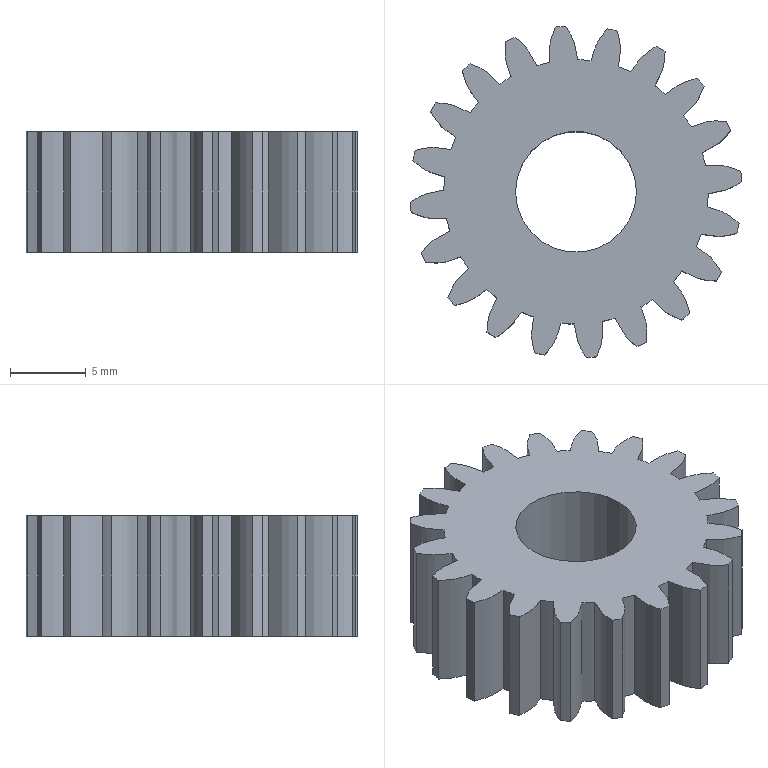Part | SolidWorks | features Boss 1, CirPattern 1, Cut 1, Extrusion 1, RefAxis 1 | 1 solid | 84 faces | box 21.958 x 21.958 x 8 mm | volume 2061 mm3 | cylinder 42 | spline 40 | plane 2 | commonest cylinder face diameters 17.5 x20 22 x20 8 x2